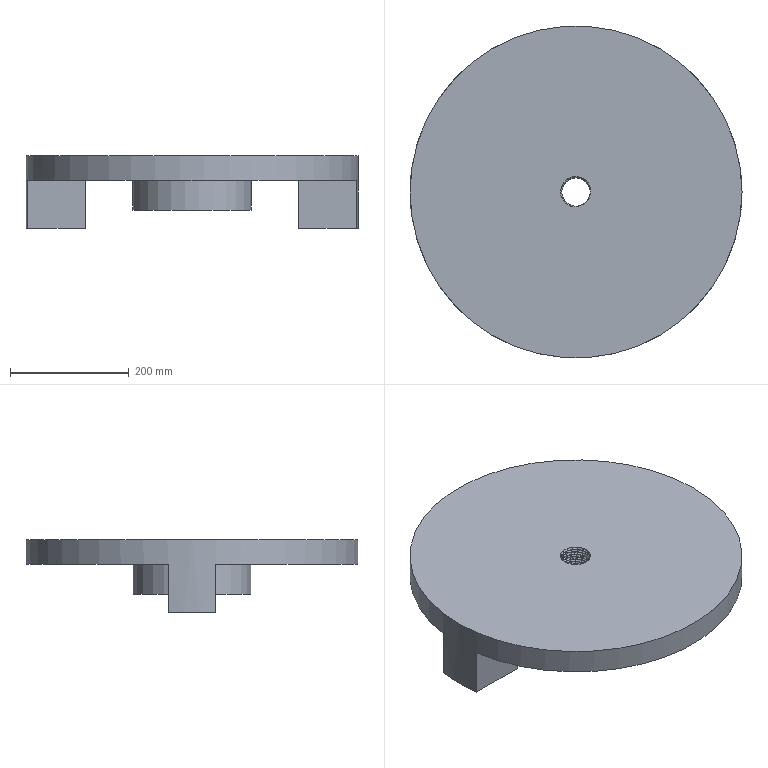Part | NX | features DATUM_CSYS 3, CYLINDER 2, EXTRUDE 2, SKETCH 2, HELIX 1, SWP104 1 | 1 solid | 336 faces | box 560 x 560 x 123 mm | volume 13014650 mm3 | torus 321 | plane 12 | cylinder 3 | commonest cylinder face diameters 48 x1 200 x1 560 x1